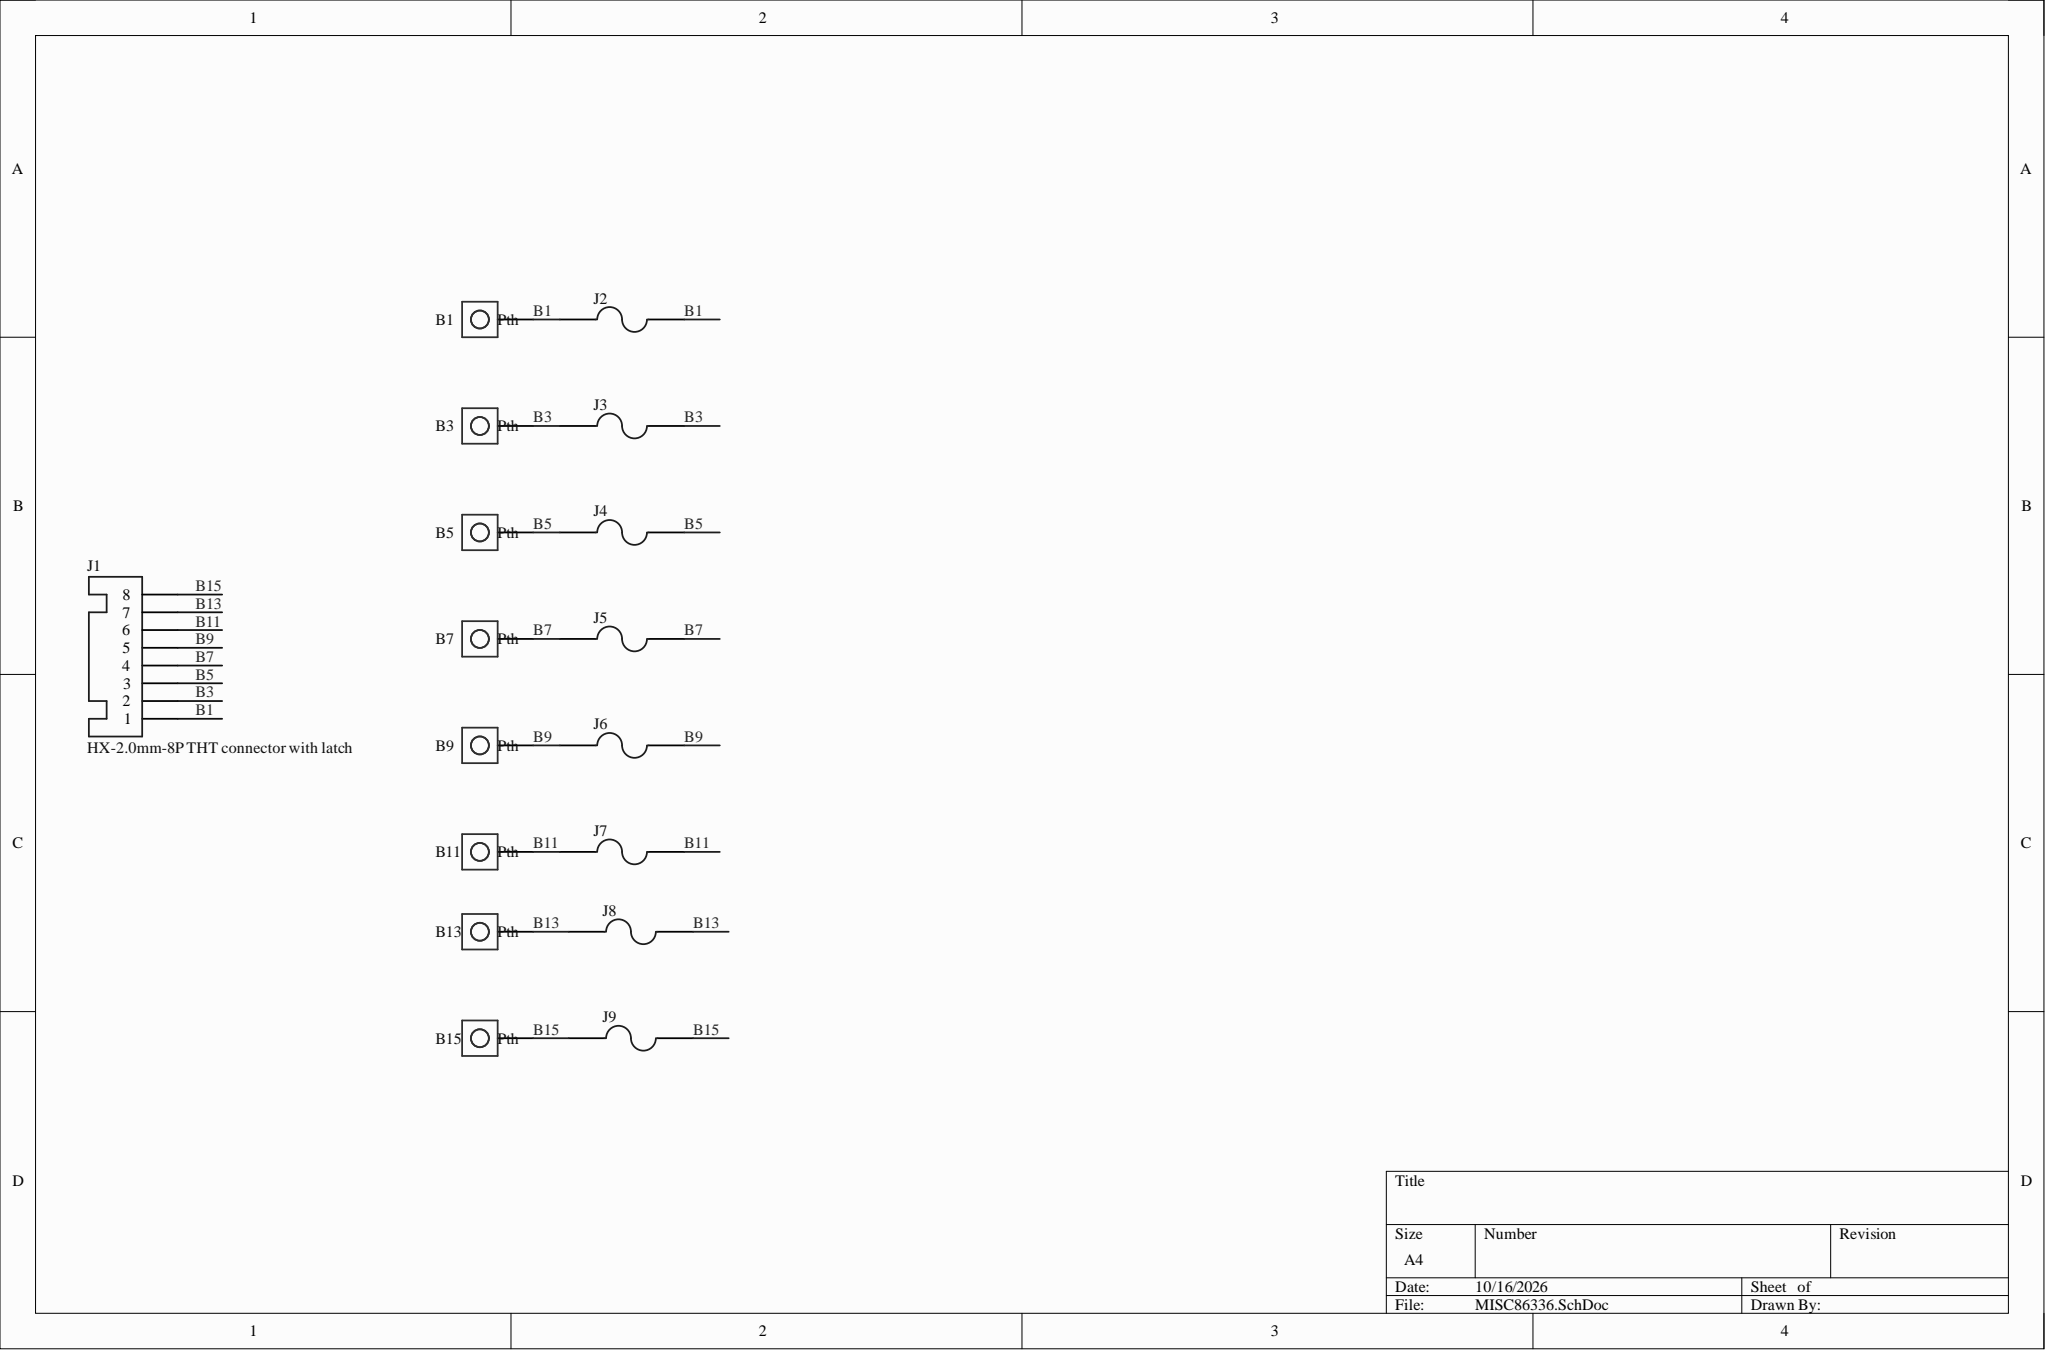Circuit board | Altium Designer | 17 parts | 8 nets
Bill of materials:
Comment,Description,Designator,Footprint,LibRef,Quantity
"Pth","Through-hole pad","B1, B3, B5, B7, B9, B11, B13, B15","55*10*1MM","Pth","8"
"HX-2.0mm-8P THT connector with latch","HX-2.0mm-8P THT connector with latch","J1","HX2.0-8P","HX-2.0mm-8P直插带扣","1"
"FPC","","J2, J3, J4, J5, J6, J7, J8, J9","异形电阻","FPC","8"
Netlist (Protel format):
[
B1
55*10*1MM
Pth



]
[
B3
55*10*1MM
Pth



]
[
B5
55*10*1MM
Pth



]
[
B7
55*10*1MM
Pth



]
[
B9
55*10*1MM
Pth



]
[
B11
55*10*1MM
Pth



]
[
B13
55*10*1MM
Pth



]
[
B15
55*10*1MM
Pth



]
[
J1
HX2.0-8P
HX-2.0mm-8P THT connector with latch



]
[
J2
异形电阻
FPC



]
[
J3
异形电阻
FPC



]
[
J4
异形电阻
FPC



]
[
J5
异形电阻
FPC



]
[
J6
异形电阻
FPC



]
[
J7
异形电阻
FPC



]
[
J8
异形电阻
FPC



]
[
J9
异形电阻
FPC



]
(
B15
B15-1
J1-8
J9-1
J9-2
)
(
B13
B13-1
J1-7
J8-1
J8-2
)
(
B11
B11-1
J1-6
J7-1
J7-2
)
(
B9
B9-1
J1-5
J6-1
J6-2
)
(
B7
B7-1
J1-4
J5-1
J5-2
)
(
B5
B5-1
J1-3
J4-1
J4-2
)
(
B3
B3-1
J1-2
J3-1
J3-2
)
(
B1
B1-1
J1-1
J2-1
J2-2
)